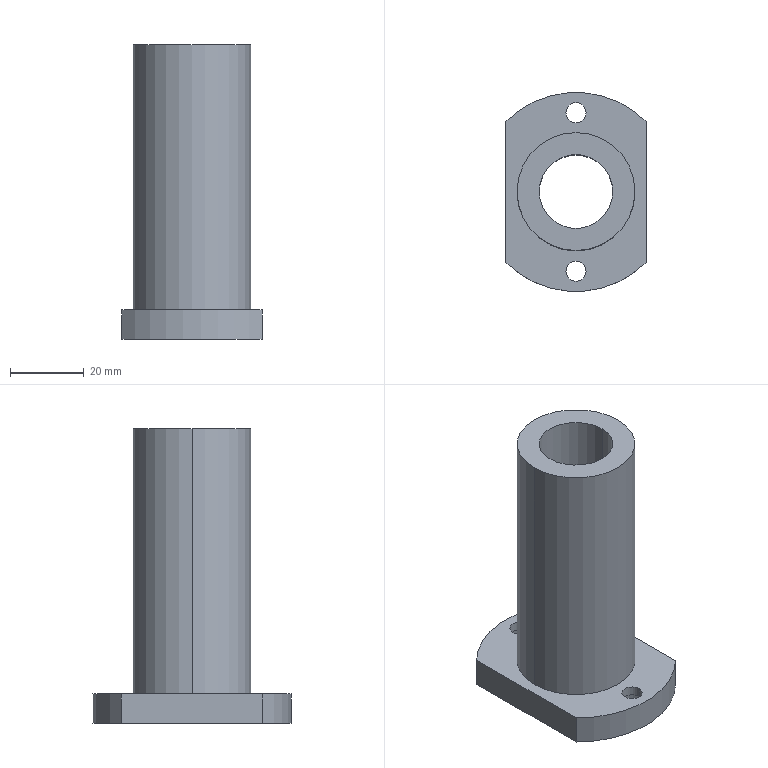Part | STEP file | Flange linear bearing | 1 solid | 21 faces | box 38 x 54 x 80 mm | volume 46738 mm3 | cylinder 14 | plane 7 | commonest cylinder face diameters 5.5 x4 10 x4 20 x2 32 x2 54 x2